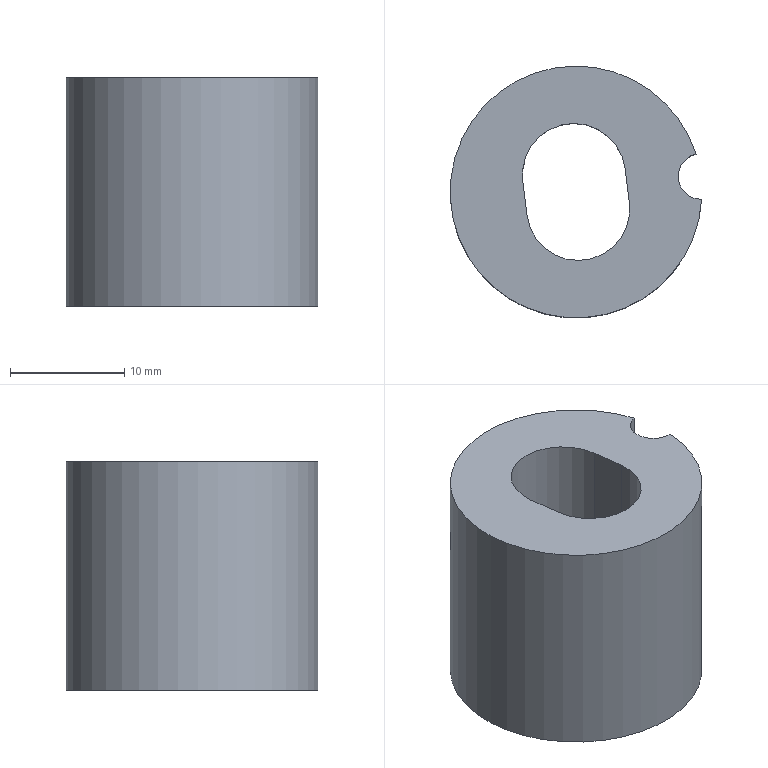Part | NX | features EKDE 22-20-12.00-9.000 2 | 1 solid | 10 faces | box 21.981 x 22 x 20 mm | volume 4748 mm3 | plane 5 | cylinder 5 | commonest cylinder face diameters 9 x2 4 x1 14.6 x1 22 x1
STEP:
#1=CARTESIAN_POINT('',(616.793,-37.978,-15.));
#2=VERTEX_POINT('',#1);
#3=CARTESIAN_POINT('',(616.3,-34.025,-15.));
#4=VERTEX_POINT('',#3);
#5=CARTESIAN_POINT('',(616.727,-35.979,-15.));
#6=DIRECTION('',(0.,0.,-1.));
#7=DIRECTION('',(1.,0.,0.));
#8=AXIS2_PLACEMENT_3D('',#5,#6,#7);
#9=CIRCLE('',#8,2.);
#10=EDGE_CURVE('',#2,#4,#9,.T.);
#11=ORIENTED_EDGE('',*,*,#10,.T.);
#12=CARTESIAN_POINT('',(605.812,-37.339,-15.));
#13=DIRECTION('',(0.,0.,-1.));
#14=DIRECTION('',(1.,0.,0.));
#15=AXIS2_PLACEMENT_3D('',#12,#13,#14);
#16=CIRCLE('',#15,11.);
#17=EDGE_CURVE('',#2,#4,#16,.T.);
#18=ORIENTED_EDGE('',*,*,#17,.F.);
#19=EDGE_LOOP('',(#11,#18));
#20=FACE_BOUND('',#19,.T.);
#21=CARTESIAN_POINT('',(610.462,-38.271,-15.));
#22=VERTEX_POINT('',#21);
#23=CARTESIAN_POINT('',(610.092,-35.294,-15.));
#24=VERTEX_POINT('',#23);
#25=CARTESIAN_POINT('',(610.277,-36.783,-15.));
#26=DIRECTION('',(-0.1236,0.9923,0.));
#27=VECTOR('',#26,1000.);
#28=LINE('',#25,#27);
#29=EDGE_CURVE('',#22,#24,#28,.T.);
#30=ORIENTED_EDGE('',*,*,#29,.F.);
#31=CARTESIAN_POINT('',(601.531,-39.384,-15.));
#32=VERTEX_POINT('',#31);
#33=CARTESIAN_POINT('',(605.997,-38.828,-15.));
#34=DIRECTION('',(0.,0.,1.));
#35=DIRECTION('',(-1.,0.,0.));
#36=AXIS2_PLACEMENT_3D('',#33,#34,#35);
#37=CIRCLE('',#36,4.5);
#38=EDGE_CURVE('',#22,#32,#37,.F.);
#39=ORIENTED_EDGE('',*,*,#38,.T.);
#40=CARTESIAN_POINT('',(601.161,-36.407,-15.));
#41=VERTEX_POINT('',#40);
#42=CARTESIAN_POINT('',(601.346,-37.896,-15.));
#43=DIRECTION('',(-0.1236,0.9923,0.));
#44=VECTOR('',#43,1000.);
#45=LINE('',#42,#44);
#46=EDGE_CURVE('',#32,#41,#45,.T.);
#47=ORIENTED_EDGE('',*,*,#46,.T.);
#48=CARTESIAN_POINT('',(605.626,-35.851,-15.));
#49=DIRECTION('',(0.,0.,1.));
#50=DIRECTION('',(-1.,0.,0.));
#51=AXIS2_PLACEMENT_3D('',#48,#49,#50);
#52=CIRCLE('',#51,4.5);
#53=EDGE_CURVE('',#41,#24,#52,.F.);
#54=ORIENTED_EDGE('',*,*,#53,.T.);
#55=EDGE_LOOP('',(#30,#39,#47,#54));
#56=FACE_BOUND('',#55,.T.);
#57=CARTESIAN_POINT('',(605.812,-37.339,-15.));
#58=DIRECTION('',(0.,0.,1.));
#59=DIRECTION('',(-1.,0.,0.));
#60=AXIS2_PLACEMENT_3D('',#57,#58,#59);
#61=PLANE('',#60);
#62=ADVANCED_FACE('',(#20,#56),#61,.T.);
#63=CARTESIAN_POINT('',(616.3,-34.025,-35.));
#64=VERTEX_POINT('',#63);
#65=CARTESIAN_POINT('',(616.793,-37.978,-35.));
#66=VERTEX_POINT('',#65);
#67=CARTESIAN_POINT('',(616.727,-35.979,-35.));
#68=DIRECTION('',(0.,0.,1.));
#69=DIRECTION('',(-1.,0.,0.));
#70=AXIS2_PLACEMENT_3D('',#67,#68,#69);
#71=CIRCLE('',#70,2.);
#72=EDGE_CURVE('',#64,#66,#71,.T.);
#73=ORIENTED_EDGE('',*,*,#72,.T.);
#74=CARTESIAN_POINT('',(605.812,-37.339,-35.));
#75=DIRECTION('',(0.,0.,1.));
#76=DIRECTION('',(-1.,0.,0.));
#77=AXIS2_PLACEMENT_3D('',#74,#75,#76);
#78=CIRCLE('',#77,11.);
#79=EDGE_CURVE('',#64,#66,#78,.T.);
#80=ORIENTED_EDGE('',*,*,#79,.F.);
#81=EDGE_LOOP('',(#73,#80));
#82=FACE_BOUND('',#81,.T.);
#83=CARTESIAN_POINT('',(613.112,-37.339,-35.));
#84=VERTEX_POINT('',#83);
#85=CARTESIAN_POINT('',(605.812,-37.339,-35.));
#86=DIRECTION('',(0.,0.,-1.));
#87=DIRECTION('',(1.,0.,0.));
#88=AXIS2_PLACEMENT_3D('',#85,#86,#87);
#89=CIRCLE('',#88,7.3);
#90=EDGE_CURVE('',#84,#84,#89,.T.);
#91=ORIENTED_EDGE('',*,*,#90,.F.);
#92=EDGE_LOOP('',(#91));
#93=FACE_BOUND('',#92,.T.);
#94=CARTESIAN_POINT('',(605.812,-37.339,-35.));
#95=DIRECTION('',(0.,0.,-1.));
#96=DIRECTION('',(1.,0.,0.));
#97=AXIS2_PLACEMENT_3D('',#94,#95,#96);
#98=PLANE('',#97);
#99=ADVANCED_FACE('',(#82,#93),#98,.T.);
#100=CARTESIAN_POINT('',(616.793,-37.978,-25.));
#101=DIRECTION('',(0.,0.,-1.));
#102=VECTOR('',#101,1000.);
#103=LINE('',#100,#102);
#104=EDGE_CURVE('',#2,#66,#103,.T.);
#105=ORIENTED_EDGE('',*,*,#104,.F.);
#106=ORIENTED_EDGE('',*,*,#17,.T.);
#107=CARTESIAN_POINT('',(616.3,-34.025,-25.));
#108=DIRECTION('',(0.,0.,-1.));
#109=VECTOR('',#108,1000.);
#110=LINE('',#107,#109);
#111=EDGE_CURVE('',#64,#4,#110,.F.);
#112=ORIENTED_EDGE('',*,*,#111,.F.);
#113=ORIENTED_EDGE('',*,*,#79,.T.);
#114=EDGE_LOOP('',(#105,#106,#112,#113));
#115=FACE_BOUND('',#114,.T.);
#116=CARTESIAN_POINT('',(605.812,-37.339,-15.));
#117=DIRECTION('',(0.,0.,-1.));
#118=DIRECTION('',(1.,0.,0.));
#119=AXIS2_PLACEMENT_3D('',#116,#117,#118);
#120=CYLINDRICAL_SURFACE('',#119,11.);
#121=ADVANCED_FACE('',(#115),#120,.T.);
#122=CARTESIAN_POINT('',(601.531,-39.384,-23.));
#123=VERTEX_POINT('',#122);
#124=CARTESIAN_POINT('',(610.462,-38.271,-23.));
#125=VERTEX_POINT('',#124);
#126=CARTESIAN_POINT('',(605.997,-38.828,-23.));
#127=DIRECTION('',(0.,0.,1.));
#128=DIRECTION('',(-1.,0.,0.));
#129=AXIS2_PLACEMENT_3D('',#126,#127,#128);
#130=CIRCLE('',#129,4.5);
#131=EDGE_CURVE('',#123,#125,#130,.T.);
#132=ORIENTED_EDGE('',*,*,#131,.F.);
#133=CARTESIAN_POINT('',(601.531,-39.384,-9.));
#134=DIRECTION('',(0.,0.,-1.));
#135=VECTOR('',#134,1000.);
#136=LINE('',#133,#135);
#137=EDGE_CURVE('',#32,#123,#136,.T.);
#138=ORIENTED_EDGE('',*,*,#137,.F.);
#139=ORIENTED_EDGE('',*,*,#38,.F.);
#140=CARTESIAN_POINT('',(610.462,-38.271,-9.));
#141=DIRECTION('',(0.,0.,-1.));
#142=VECTOR('',#141,1000.);
#143=LINE('',#140,#142);
#144=EDGE_CURVE('',#22,#125,#143,.T.);
#145=ORIENTED_EDGE('',*,*,#144,.T.);
#146=EDGE_LOOP('',(#132,#138,#139,#145));
#147=FACE_BOUND('',#146,.T.);
#148=CARTESIAN_POINT('',(605.997,-38.828,-9.));
#149=DIRECTION('',(0.,0.,-1.));
#150=DIRECTION('',(1.,0.,0.));
#151=AXIS2_PLACEMENT_3D('',#148,#149,#150);
#152=CYLINDRICAL_SURFACE('',#151,4.5);
#153=ADVANCED_FACE('',(#147),#152,.F.);
#154=CARTESIAN_POINT('',(610.092,-35.294,-23.));
#155=VERTEX_POINT('',#154);
#156=CARTESIAN_POINT('',(610.092,-35.294,-9.));
#157=DIRECTION('',(0.,0.,-1.));
#158=VECTOR('',#157,1000.);
#159=LINE('',#156,#158);
#160=EDGE_CURVE('',#24,#155,#159,.T.);
#161=ORIENTED_EDGE('',*,*,#160,.T.);
#162=CARTESIAN_POINT('',(610.092,-35.294,-23.));
#163=DIRECTION('',(0.1236,-0.9923,0.));
#164=VECTOR('',#163,1000.);
#165=LINE('',#162,#164);
#166=EDGE_CURVE('',#155,#125,#165,.T.);
#167=ORIENTED_EDGE('',*,*,#166,.T.);
#168=ORIENTED_EDGE('',*,*,#144,.F.);
#169=ORIENTED_EDGE('',*,*,#29,.T.);
#170=EDGE_LOOP('',(#161,#167,#168,#169));
#171=FACE_BOUND('',#170,.T.);
#172=CARTESIAN_POINT('',(610.092,-35.294,-9.));
#173=DIRECTION('',(0.9923,0.1236,0.));
#174=DIRECTION('',(-0.1236,0.9923,0.));
#175=AXIS2_PLACEMENT_3D('',#172,#173,#174);
#176=PLANE('',#175);
#177=ADVANCED_FACE('',(#171),#176,.F.);
#178=CARTESIAN_POINT('',(601.161,-36.407,-23.));
#179=VERTEX_POINT('',#178);
#180=CARTESIAN_POINT('',(605.626,-35.851,-23.));
#181=DIRECTION('',(0.,0.,1.));
#182=DIRECTION('',(-1.,0.,0.));
#183=AXIS2_PLACEMENT_3D('',#180,#181,#182);
#184=CIRCLE('',#183,4.5);
#185=EDGE_CURVE('',#155,#179,#184,.T.);
#186=ORIENTED_EDGE('',*,*,#185,.F.);
#187=ORIENTED_EDGE('',*,*,#160,.F.);
#188=ORIENTED_EDGE('',*,*,#53,.F.);
#189=CARTESIAN_POINT('',(601.161,-36.407,-9.));
#190=DIRECTION('',(0.,0.,-1.));
#191=VECTOR('',#190,1000.);
#192=LINE('',#189,#191);
#193=EDGE_CURVE('',#41,#179,#192,.T.);
#194=ORIENTED_EDGE('',*,*,#193,.T.);
#195=EDGE_LOOP('',(#186,#187,#188,#194));
#196=FACE_BOUND('',#195,.T.);
#197=CARTESIAN_POINT('',(605.626,-35.851,-9.));
#198=DIRECTION('',(0.,0.,-1.));
#199=DIRECTION('',(1.,0.,0.));
#200=AXIS2_PLACEMENT_3D('',#197,#198,#199);
#201=CYLINDRICAL_SURFACE('',#200,4.5);
#202=ADVANCED_FACE('',(#196),#201,.F.);
#203=CARTESIAN_POINT('',(601.161,-36.407,-23.));
#204=DIRECTION('',(0.1236,-0.9923,0.));
#205=VECTOR('',#204,1000.);
#206=LINE('',#203,#205);
#207=EDGE_CURVE('',#179,#123,#206,.T.);
#208=ORIENTED_EDGE('',*,*,#207,.F.);
#209=ORIENTED_EDGE('',*,*,#193,.F.);
#210=ORIENTED_EDGE('',*,*,#46,.F.);
#211=ORIENTED_EDGE('',*,*,#137,.T.);
#212=EDGE_LOOP('',(#208,#209,#210,#211));
#213=FACE_BOUND('',#212,.T.);
#214=CARTESIAN_POINT('',(601.161,-36.407,-9.));
#215=DIRECTION('',(0.9923,0.1236,0.));
#216=DIRECTION('',(-0.1236,0.9923,0.));
#217=AXIS2_PLACEMENT_3D('',#214,#215,#216);
#218=PLANE('',#217);
#219=ADVANCED_FACE('',(#213),#218,.T.);
#220=ORIENTED_EDGE('',*,*,#131,.T.);
#221=ORIENTED_EDGE('',*,*,#166,.F.);
#222=ORIENTED_EDGE('',*,*,#185,.T.);
#223=ORIENTED_EDGE('',*,*,#207,.T.);
#224=EDGE_LOOP('',(#220,#221,#222,#223));
#225=FACE_BOUND('',#224,.T.);
#226=CARTESIAN_POINT('',(613.112,-37.339,-23.));
#227=VERTEX_POINT('',#226);
#228=CARTESIAN_POINT('',(605.812,-37.339,-23.));
#229=DIRECTION('',(0.,0.,-1.));
#230=DIRECTION('',(1.,0.,0.));
#231=AXIS2_PLACEMENT_3D('',#228,#229,#230);
#232=CIRCLE('',#231,7.3);
#233=EDGE_CURVE('',#227,#227,#232,.T.);
#234=ORIENTED_EDGE('',*,*,#233,.T.);
#235=EDGE_LOOP('',(#234));
#236=FACE_BOUND('',#235,.T.);
#237=CARTESIAN_POINT('',(605.812,-37.339,-23.));
#238=DIRECTION('',(0.,0.,1.));
#239=DIRECTION('',(-1.,0.,0.));
#240=AXIS2_PLACEMENT_3D('',#237,#238,#239);
#241=PLANE('',#240);
#242=ADVANCED_FACE('',(#225,#236),#241,.F.);
#243=ORIENTED_EDGE('',*,*,#90,.T.);
#244=EDGE_LOOP('',(#243));
#245=FACE_BOUND('',#244,.T.);
#246=ORIENTED_EDGE('',*,*,#233,.F.);
#247=EDGE_LOOP('',(#246));
#248=FACE_BOUND('',#247,.T.);
#249=CARTESIAN_POINT('',(605.812,-37.339,-23.));
#250=DIRECTION('',(0.,0.,-1.));
#251=DIRECTION('',(1.,0.,0.));
#252=AXIS2_PLACEMENT_3D('',#249,#250,#251);
#253=CYLINDRICAL_SURFACE('',#252,7.3);
#254=ADVANCED_FACE('',(#245,#248),#253,.F.);
#255=ORIENTED_EDGE('',*,*,#104,.T.);
#256=ORIENTED_EDGE('',*,*,#72,.F.);
#257=ORIENTED_EDGE('',*,*,#111,.T.);
#258=ORIENTED_EDGE('',*,*,#10,.F.);
#259=EDGE_LOOP('',(#255,#256,#257,#258));
#260=FACE_BOUND('',#259,.T.);
#261=CARTESIAN_POINT('',(616.727,-35.979,-15.));
#262=DIRECTION('',(0.,0.,-1.));
#263=DIRECTION('',(1.,0.,0.));
#264=AXIS2_PLACEMENT_3D('',#261,#262,#263);
#265=CYLINDRICAL_SURFACE('',#264,2.);
#266=ADVANCED_FACE('',(#260),#265,.F.);
#267=CLOSED_SHELL('',(#62,#99,#121,#153,#177,#202,#219,#242,#254,#266));
#268=MANIFOLD_SOLID_BREP('',#267);
#269=(LENGTH_UNIT()NAMED_UNIT(*)SI_UNIT(.MILLI.,.METRE.));
#270=UNCERTAINTY_MEASURE_WITH_UNIT(LENGTH_MEASURE(0.00001),#269,'','');
#271=(NAMED_UNIT(*)PLANE_ANGLE_UNIT()SI_UNIT($,.RADIAN.));
#272=(NAMED_UNIT(*)SI_UNIT($,.STERADIAN.)SOLID_ANGLE_UNIT());
#273=(GEOMETRIC_REPRESENTATION_CONTEXT(3)GLOBAL_UNCERTAINTY_ASSIGNED_CONTEXT((#270))GLOBAL_UNIT_ASSIGNED_CONTEXT((#269,#271,#272))REPRESENTATION_CONTEXT('',''));
#274=ADVANCED_BREP_SHAPE_REPRESENTATION('',(#268),#273);